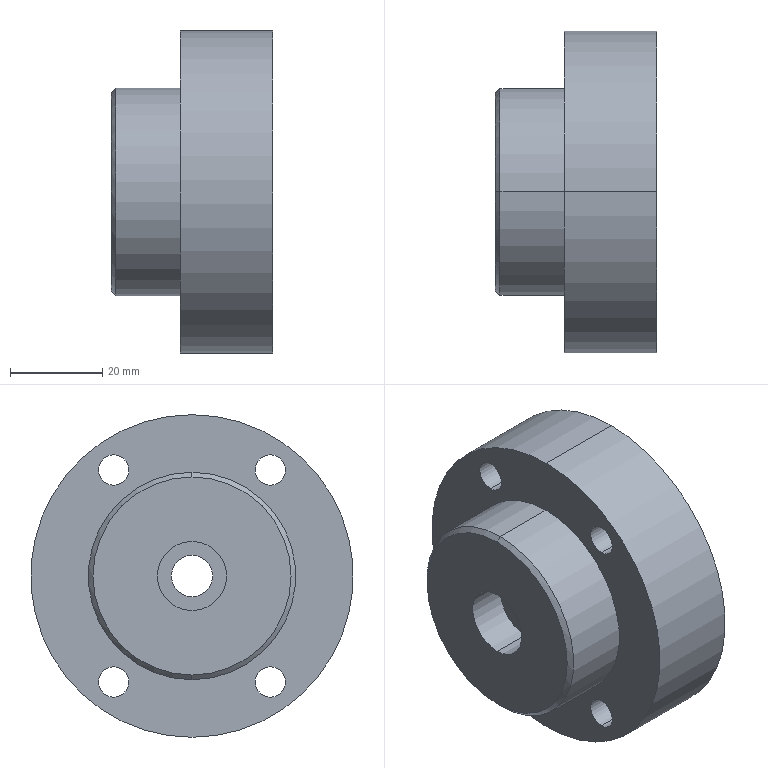Part | SolidWorks | features BaseBody 1 | 1 solid | 39 faces | box 35 x 70 x 70 mm | volume 84677 mm3 | cylinder 26 | plane 9 | cone 4 | commonest cylinder face diameters 6.6 x8 11 x8 9 x2 15 x2 25 x2 45 x2
STEP:
#1=CARTESIAN_POINT('',(8.6,0.,-7.5));
#2=VERTEX_POINT('',#1);
#3=CARTESIAN_POINT('',(8.6,0.,7.5));
#4=VERTEX_POINT('',#3);
#5=CARTESIAN_POINT('',(8.6,0.,0.));
#6=DIRECTION('',(-1.,0.,0.));
#7=DIRECTION('',(0.,0.,1.));
#8=AXIS2_PLACEMENT_3D('',#5,#6,#7);
#9=CIRCLE('',#8,7.5);
#10=EDGE_CURVE('',#2,#4,#9,.T.);
#11=ORIENTED_EDGE('',*,*,#10,.F.);
#12=CARTESIAN_POINT('',(0.,0.,-7.5));
#13=VERTEX_POINT('',#12);
#14=CARTESIAN_POINT('',(0.,0.,-7.5));
#15=DIRECTION('',(-1.,0.,0.));
#16=VECTOR('',#15,1000.);
#17=LINE('',#14,#16);
#18=EDGE_CURVE('',#2,#13,#17,.T.);
#19=ORIENTED_EDGE('',*,*,#18,.T.);
#20=CARTESIAN_POINT('',(0.,0.,7.5));
#21=VERTEX_POINT('',#20);
#22=CARTESIAN_POINT('',(0.,0.,0.));
#23=DIRECTION('',(-1.,0.,0.));
#24=DIRECTION('',(0.,0.,1.));
#25=AXIS2_PLACEMENT_3D('',#22,#23,#24);
#26=CIRCLE('',#25,7.5);
#27=EDGE_CURVE('',#13,#21,#26,.T.);
#28=ORIENTED_EDGE('',*,*,#27,.T.);
#29=CARTESIAN_POINT('',(0.,0.,7.5));
#30=DIRECTION('',(-1.,0.,0.));
#31=VECTOR('',#30,1000.);
#32=LINE('',#29,#31);
#33=EDGE_CURVE('',#4,#21,#32,.T.);
#34=ORIENTED_EDGE('',*,*,#33,.F.);
#35=EDGE_LOOP('',(#11,#19,#28,#34));
#36=FACE_OUTER_BOUND('',#35,.T.);
#37=CARTESIAN_POINT('',(0.,0.,0.));
#38=DIRECTION('',(-1.,0.,0.));
#39=DIRECTION('',(0.,0.,1.));
#40=AXIS2_PLACEMENT_3D('',#37,#38,#39);
#41=CYLINDRICAL_SURFACE('',#40,7.5);
#42=ADVANCED_FACE('',(#36),#41,.F.);
#43=CARTESIAN_POINT('',(15.,0.,-4.5));
#44=VERTEX_POINT('',#43);
#45=CARTESIAN_POINT('',(15.,0.,4.5));
#46=VERTEX_POINT('',#45);
#47=CARTESIAN_POINT('',(15.,0.,0.));
#48=DIRECTION('',(-1.,0.,0.));
#49=DIRECTION('',(0.,0.,1.));
#50=AXIS2_PLACEMENT_3D('',#47,#48,#49);
#51=CIRCLE('',#50,4.5);
#52=EDGE_CURVE('',#44,#46,#51,.T.);
#53=ORIENTED_EDGE('',*,*,#52,.F.);
#54=CARTESIAN_POINT('',(8.6,0.,-4.5));
#55=VERTEX_POINT('',#54);
#56=CARTESIAN_POINT('',(0.,0.,-4.5));
#57=DIRECTION('',(-1.,0.,0.));
#58=VECTOR('',#57,1000.);
#59=LINE('',#56,#58);
#60=EDGE_CURVE('',#44,#55,#59,.T.);
#61=ORIENTED_EDGE('',*,*,#60,.T.);
#62=CARTESIAN_POINT('',(8.6,0.,4.5));
#63=VERTEX_POINT('',#62);
#64=CARTESIAN_POINT('',(8.6,0.,0.));
#65=DIRECTION('',(-1.,0.,0.));
#66=DIRECTION('',(0.,0.,1.));
#67=AXIS2_PLACEMENT_3D('',#64,#65,#66);
#68=CIRCLE('',#67,4.5);
#69=EDGE_CURVE('',#55,#63,#68,.T.);
#70=ORIENTED_EDGE('',*,*,#69,.T.);
#71=CARTESIAN_POINT('',(0.,0.,4.5));
#72=DIRECTION('',(-1.,0.,0.));
#73=VECTOR('',#72,1000.);
#74=LINE('',#71,#73);
#75=EDGE_CURVE('',#46,#63,#74,.T.);
#76=ORIENTED_EDGE('',*,*,#75,.F.);
#77=EDGE_LOOP('',(#53,#61,#70,#76));
#78=FACE_OUTER_BOUND('',#77,.T.);
#79=CARTESIAN_POINT('',(0.,0.,0.));
#80=DIRECTION('',(-1.,0.,0.));
#81=DIRECTION('',(0.,0.,1.));
#82=AXIS2_PLACEMENT_3D('',#79,#80,#81);
#83=CYLINDRICAL_SURFACE('',#82,4.5);
#84=ADVANCED_FACE('',(#78),#83,.F.);
#85=CARTESIAN_POINT('',(0.,0.,21.5));
#86=VERTEX_POINT('',#85);
#87=CARTESIAN_POINT('',(0.,0.,-21.5));
#88=VERTEX_POINT('',#87);
#89=CARTESIAN_POINT('',(0.,0.,0.));
#90=DIRECTION('',(-1.,0.,0.));
#91=DIRECTION('',(0.,0.,-1.));
#92=AXIS2_PLACEMENT_3D('',#89,#90,#91);
#93=CIRCLE('',#92,21.5);
#94=EDGE_CURVE('',#86,#88,#93,.T.);
#95=ORIENTED_EDGE('',*,*,#94,.F.);
#96=CARTESIAN_POINT('',(1.,0.,22.5));
#97=VERTEX_POINT('',#96);
#98=CARTESIAN_POINT('',(1.,0.,22.5));
#99=DIRECTION('',(0.7071,0.,0.7071));
#100=VECTOR('',#99,1000.);
#101=LINE('',#98,#100);
#102=EDGE_CURVE('',#86,#97,#101,.T.);
#103=ORIENTED_EDGE('',*,*,#102,.T.);
#104=CARTESIAN_POINT('',(1.,0.,-22.5));
#105=VERTEX_POINT('',#104);
#106=CARTESIAN_POINT('',(1.,0.,0.));
#107=DIRECTION('',(1.,0.,0.));
#108=DIRECTION('',(0.,0.,-1.));
#109=AXIS2_PLACEMENT_3D('',#106,#107,#108);
#110=CIRCLE('',#109,22.5);
#111=EDGE_CURVE('',#105,#97,#110,.T.);
#112=ORIENTED_EDGE('',*,*,#111,.F.);
#113=CARTESIAN_POINT('',(1.,0.,-22.5));
#114=DIRECTION('',(0.7071,0.,-0.7071));
#115=VECTOR('',#114,1000.);
#116=LINE('',#113,#115);
#117=EDGE_CURVE('',#88,#105,#116,.T.);
#118=ORIENTED_EDGE('',*,*,#117,.F.);
#119=EDGE_LOOP('',(#95,#103,#112,#118));
#120=FACE_OUTER_BOUND('',#119,.T.);
#121=CARTESIAN_POINT('',(1.,0.,0.));
#122=DIRECTION('',(1.,0.,0.));
#123=DIRECTION('',(0.,0.,-1.));
#124=AXIS2_PLACEMENT_3D('',#121,#122,#123);
#125=CONICAL_SURFACE('',#124,22.5,0.7854);
#126=ADVANCED_FACE('',(#120),#125,.T.);
#127=CARTESIAN_POINT('',(34.,0.,12.5));
#128=VERTEX_POINT('',#127);
#129=CARTESIAN_POINT('',(34.,0.,-12.5));
#130=VERTEX_POINT('',#129);
#131=CARTESIAN_POINT('',(34.,0.,0.));
#132=DIRECTION('',(1.,0.,0.));
#133=DIRECTION('',(0.,0.,-1.));
#134=AXIS2_PLACEMENT_3D('',#131,#132,#133);
#135=CIRCLE('',#134,12.5);
#136=EDGE_CURVE('',#128,#130,#135,.T.);
#137=ORIENTED_EDGE('',*,*,#136,.F.);
#138=CARTESIAN_POINT('',(35.,0.,13.5));
#139=VERTEX_POINT('',#138);
#140=CARTESIAN_POINT('',(35.,0.,13.5));
#141=DIRECTION('',(0.7071,0.,0.7071));
#142=VECTOR('',#141,1000.);
#143=LINE('',#140,#142);
#144=EDGE_CURVE('',#128,#139,#143,.T.);
#145=ORIENTED_EDGE('',*,*,#144,.T.);
#146=CARTESIAN_POINT('',(35.,0.,-13.5));
#147=VERTEX_POINT('',#146);
#148=CARTESIAN_POINT('',(35.,0.,0.));
#149=DIRECTION('',(-1.,0.,0.));
#150=DIRECTION('',(0.,0.,-1.));
#151=AXIS2_PLACEMENT_3D('',#148,#149,#150);
#152=CIRCLE('',#151,13.5);
#153=EDGE_CURVE('',#147,#139,#152,.T.);
#154=ORIENTED_EDGE('',*,*,#153,.F.);
#155=CARTESIAN_POINT('',(35.,0.,-13.5));
#156=DIRECTION('',(0.7071,0.,-0.7071));
#157=VECTOR('',#156,1000.);
#158=LINE('',#155,#157);
#159=EDGE_CURVE('',#130,#147,#158,.T.);
#160=ORIENTED_EDGE('',*,*,#159,.F.);
#161=EDGE_LOOP('',(#137,#145,#154,#160));
#162=FACE_OUTER_BOUND('',#161,.T.);
#163=CARTESIAN_POINT('',(35.,0.,0.));
#164=DIRECTION('',(1.,0.,0.));
#165=DIRECTION('',(0.,0.,-1.));
#166=AXIS2_PLACEMENT_3D('',#163,#164,#165);
#167=CONICAL_SURFACE('',#166,13.5,0.7854);
#168=ADVANCED_FACE('',(#162),#167,.F.);
#169=CARTESIAN_POINT('',(28.6,17.,28.5));
#170=VERTEX_POINT('',#169);
#171=CARTESIAN_POINT('',(28.6,17.,17.5));
#172=VERTEX_POINT('',#171);
#173=CARTESIAN_POINT('',(28.6,17.,23.));
#174=DIRECTION('',(1.,0.,0.));
#175=DIRECTION('',(0.,0.,-1.));
#176=AXIS2_PLACEMENT_3D('',#173,#174,#175);
#177=CIRCLE('',#176,5.5);
#178=EDGE_CURVE('',#170,#172,#177,.T.);
#179=ORIENTED_EDGE('',*,*,#178,.F.);
#180=CARTESIAN_POINT('',(35.,17.,28.5));
#181=VERTEX_POINT('',#180);
#182=CARTESIAN_POINT('',(35.,17.,28.5));
#183=DIRECTION('',(1.,0.,0.));
#184=VECTOR('',#183,1000.);
#185=LINE('',#182,#184);
#186=EDGE_CURVE('',#170,#181,#185,.T.);
#187=ORIENTED_EDGE('',*,*,#186,.T.);
#188=CARTESIAN_POINT('',(35.,17.,17.5));
#189=VERTEX_POINT('',#188);
#190=CARTESIAN_POINT('',(35.,17.,23.));
#191=DIRECTION('',(1.,0.,0.));
#192=DIRECTION('',(0.,0.,-1.));
#193=AXIS2_PLACEMENT_3D('',#190,#191,#192);
#194=CIRCLE('',#193,5.5);
#195=EDGE_CURVE('',#181,#189,#194,.T.);
#196=ORIENTED_EDGE('',*,*,#195,.T.);
#197=CARTESIAN_POINT('',(35.,17.,17.5));
#198=DIRECTION('',(1.,0.,0.));
#199=VECTOR('',#198,1000.);
#200=LINE('',#197,#199);
#201=EDGE_CURVE('',#172,#189,#200,.T.);
#202=ORIENTED_EDGE('',*,*,#201,.F.);
#203=EDGE_LOOP('',(#179,#187,#196,#202));
#204=FACE_OUTER_BOUND('',#203,.T.);
#205=CARTESIAN_POINT('',(35.,17.,23.));
#206=DIRECTION('',(1.,0.,0.));
#207=DIRECTION('',(0.,0.,-1.));
#208=AXIS2_PLACEMENT_3D('',#205,#206,#207);
#209=CYLINDRICAL_SURFACE('',#208,5.5);
#210=ADVANCED_FACE('',(#204),#209,.F.);
#211=CARTESIAN_POINT('',(15.,17.,26.3));
#212=VERTEX_POINT('',#211);
#213=CARTESIAN_POINT('',(15.,17.,19.7));
#214=VERTEX_POINT('',#213);
#215=CARTESIAN_POINT('',(15.,17.,23.));
#216=DIRECTION('',(1.,0.,0.));
#217=DIRECTION('',(0.,0.,-1.));
#218=AXIS2_PLACEMENT_3D('',#215,#216,#217);
#219=CIRCLE('',#218,3.3);
#220=EDGE_CURVE('',#212,#214,#219,.T.);
#221=ORIENTED_EDGE('',*,*,#220,.F.);
#222=CARTESIAN_POINT('',(28.6,17.,26.3));
#223=VERTEX_POINT('',#222);
#224=CARTESIAN_POINT('',(35.,17.,26.3));
#225=DIRECTION('',(1.,0.,0.));
#226=VECTOR('',#225,1000.);
#227=LINE('',#224,#226);
#228=EDGE_CURVE('',#212,#223,#227,.T.);
#229=ORIENTED_EDGE('',*,*,#228,.T.);
#230=CARTESIAN_POINT('',(28.6,17.,19.7));
#231=VERTEX_POINT('',#230);
#232=CARTESIAN_POINT('',(28.6,17.,23.));
#233=DIRECTION('',(1.,0.,0.));
#234=DIRECTION('',(0.,0.,-1.));
#235=AXIS2_PLACEMENT_3D('',#232,#233,#234);
#236=CIRCLE('',#235,3.3);
#237=EDGE_CURVE('',#223,#231,#236,.T.);
#238=ORIENTED_EDGE('',*,*,#237,.T.);
#239=CARTESIAN_POINT('',(35.,17.,19.7));
#240=DIRECTION('',(1.,0.,0.));
#241=VECTOR('',#240,1000.);
#242=LINE('',#239,#241);
#243=EDGE_CURVE('',#214,#231,#242,.T.);
#244=ORIENTED_EDGE('',*,*,#243,.F.);
#245=EDGE_LOOP('',(#221,#229,#238,#244));
#246=FACE_OUTER_BOUND('',#245,.T.);
#247=CARTESIAN_POINT('',(35.,17.,23.));
#248=DIRECTION('',(1.,0.,0.));
#249=DIRECTION('',(0.,0.,-1.));
#250=AXIS2_PLACEMENT_3D('',#247,#248,#249);
#251=CYLINDRICAL_SURFACE('',#250,3.3);
#252=ADVANCED_FACE('',(#246),#251,.F.);
#253=CARTESIAN_POINT('',(28.6,17.,-17.5));
#254=VERTEX_POINT('',#253);
#255=CARTESIAN_POINT('',(28.6,17.,-28.5));
#256=VERTEX_POINT('',#255);
#257=CARTESIAN_POINT('',(28.6,17.,-23.));
#258=DIRECTION('',(1.,0.,0.));
#259=DIRECTION('',(0.,0.,-1.));
#260=AXIS2_PLACEMENT_3D('',#257,#258,#259);
#261=CIRCLE('',#260,5.5);
#262=EDGE_CURVE('',#254,#256,#261,.T.);
#263=ORIENTED_EDGE('',*,*,#262,.F.);
#264=CARTESIAN_POINT('',(35.,17.,-17.5));
#265=VERTEX_POINT('',#264);
#266=CARTESIAN_POINT('',(35.,17.,-17.5));
#267=DIRECTION('',(1.,0.,0.));
#268=VECTOR('',#267,1000.);
#269=LINE('',#266,#268);
#270=EDGE_CURVE('',#254,#265,#269,.T.);
#271=ORIENTED_EDGE('',*,*,#270,.T.);
#272=CARTESIAN_POINT('',(35.,17.,-28.5));
#273=VERTEX_POINT('',#272);
#274=CARTESIAN_POINT('',(35.,17.,-23.));
#275=DIRECTION('',(1.,0.,0.));
#276=DIRECTION('',(0.,0.,-1.));
#277=AXIS2_PLACEMENT_3D('',#274,#275,#276);
#278=CIRCLE('',#277,5.5);
#279=EDGE_CURVE('',#265,#273,#278,.T.);
#280=ORIENTED_EDGE('',*,*,#279,.T.);
#281=CARTESIAN_POINT('',(35.,17.,-28.5));
#282=DIRECTION('',(1.,0.,0.));
#283=VECTOR('',#282,1000.);
#284=LINE('',#281,#283);
#285=EDGE_CURVE('',#256,#273,#284,.T.);
#286=ORIENTED_EDGE('',*,*,#285,.F.);
#287=EDGE_LOOP('',(#263,#271,#280,#286));
#288=FACE_OUTER_BOUND('',#287,.T.);
#289=CARTESIAN_POINT('',(35.,17.,-23.));
#290=DIRECTION('',(1.,0.,0.));
#291=DIRECTION('',(0.,0.,-1.));
#292=AXIS2_PLACEMENT_3D('',#289,#290,#291);
#293=CYLINDRICAL_SURFACE('',#292,5.5);
#294=ADVANCED_FACE('',(#288),#293,.F.);
#295=CARTESIAN_POINT('',(15.,17.,-19.7));
#296=VERTEX_POINT('',#295);
#297=CARTESIAN_POINT('',(15.,17.,-26.3));
#298=VERTEX_POINT('',#297);
#299=CARTESIAN_POINT('',(15.,17.,-23.));
#300=DIRECTION('',(1.,0.,0.));
#301=DIRECTION('',(0.,0.,-1.));
#302=AXIS2_PLACEMENT_3D('',#299,#300,#301);
#303=CIRCLE('',#302,3.3);
#304=EDGE_CURVE('',#296,#298,#303,.T.);
#305=ORIENTED_EDGE('',*,*,#304,.F.);
#306=CARTESIAN_POINT('',(28.6,17.,-19.7));
#307=VERTEX_POINT('',#306);
#308=CARTESIAN_POINT('',(35.,17.,-19.7));
#309=DIRECTION('',(1.,0.,0.));
#310=VECTOR('',#309,1000.);
#311=LINE('',#308,#310);
#312=EDGE_CURVE('',#296,#307,#311,.T.);
#313=ORIENTED_EDGE('',*,*,#312,.T.);
#314=CARTESIAN_POINT('',(28.6,17.,-26.3));
#315=VERTEX_POINT('',#314);
#316=CARTESIAN_POINT('',(28.6,17.,-23.));
#317=DIRECTION('',(1.,0.,0.));
#318=DIRECTION('',(0.,0.,-1.));
#319=AXIS2_PLACEMENT_3D('',#316,#317,#318);
#320=CIRCLE('',#319,3.3);
#321=EDGE_CURVE('',#307,#315,#320,.T.);
#322=ORIENTED_EDGE('',*,*,#321,.T.);
#323=CARTESIAN_POINT('',(35.,17.,-26.3));
#324=DIRECTION('',(1.,0.,0.));
#325=VECTOR('',#324,1000.);
#326=LINE('',#323,#325);
#327=EDGE_CURVE('',#298,#315,#326,.T.);
#328=ORIENTED_EDGE('',*,*,#327,.F.);
#329=EDGE_LOOP('',(#305,#313,#322,#328));
#330=FACE_OUTER_BOUND('',#329,.T.);
#331=CARTESIAN_POINT('',(35.,17.,-23.));
#332=DIRECTION('',(1.,0.,0.));
#333=DIRECTION('',(0.,0.,-1.));
#334=AXIS2_PLACEMENT_3D('',#331,#332,#333);
#335=CYLINDRICAL_SURFACE('',#334,3.3);
#336=ADVANCED_FACE('',(#330),#335,.F.);
#337=CARTESIAN_POINT('',(28.6,-17.,-17.5));
#338=VERTEX_POINT('',#337);
#339=CARTESIAN_POINT('',(28.6,-17.,-28.5));
#340=VERTEX_POINT('',#339);
#341=CARTESIAN_POINT('',(28.6,-17.,-23.));
#342=DIRECTION('',(1.,0.,0.));
#343=DIRECTION('',(0.,0.,-1.));
#344=AXIS2_PLACEMENT_3D('',#341,#342,#343);
#345=CIRCLE('',#344,5.5);
#346=EDGE_CURVE('',#338,#340,#345,.T.);
#347=ORIENTED_EDGE('',*,*,#346,.F.);
#348=CARTESIAN_POINT('',(35.,-17.,-17.5));
#349=VERTEX_POINT('',#348);
#350=CARTESIAN_POINT('',(35.,-17.,-17.5));
#351=DIRECTION('',(1.,0.,0.));
#352=VECTOR('',#351,1000.);
#353=LINE('',#350,#352);
#354=EDGE_CURVE('',#338,#349,#353,.T.);
#355=ORIENTED_EDGE('',*,*,#354,.T.);
#356=CARTESIAN_POINT('',(35.,-17.,-28.5));
#357=VERTEX_POINT('',#356);
#358=CARTESIAN_POINT('',(35.,-17.,-23.));
#359=DIRECTION('',(1.,0.,0.));
#360=DIRECTION('',(0.,0.,-1.));
#361=AXIS2_PLACEMENT_3D('',#358,#359,#360);
#362=CIRCLE('',#361,5.5);
#363=EDGE_CURVE('',#349,#357,#362,.T.);
#364=ORIENTED_EDGE('',*,*,#363,.T.);
#365=CARTESIAN_POINT('',(35.,-17.,-28.5));
#366=DIRECTION('',(1.,0.,0.));
#367=VECTOR('',#366,1000.);
#368=LINE('',#365,#367);
#369=EDGE_CURVE('',#340,#357,#368,.T.);
#370=ORIENTED_EDGE('',*,*,#369,.F.);
#371=EDGE_LOOP('',(#347,#355,#364,#370));
#372=FACE_OUTER_BOUND('',#371,.T.);
#373=CARTESIAN_POINT('',(35.,-17.,-23.));
#374=DIRECTION('',(1.,0.,0.));
#375=DIRECTION('',(0.,0.,-1.));
#376=AXIS2_PLACEMENT_3D('',#373,#374,#375);
#377=CYLINDRICAL_SURFACE('',#376,5.5);
#378=ADVANCED_FACE('',(#372),#377,.F.);
#379=CARTESIAN_POINT('',(15.,-17.,-19.7));
#380=VERTEX_POINT('',#379);
#381=CARTESIAN_POINT('',(15.,-17.,-26.3));
#382=VERTEX_POINT('',#381);
#383=CARTESIAN_POINT('',(15.,-17.,-23.));
#384=DIRECTION('',(1.,0.,0.));
#385=DIRECTION('',(0.,0.,-1.));
#386=AXIS2_PLACEMENT_3D('',#383,#384,#385);
#387=CIRCLE('',#386,3.3);
#388=EDGE_CURVE('',#380,#382,#387,.T.);
#389=ORIENTED_EDGE('',*,*,#388,.F.);
#390=CARTESIAN_POINT('',(28.6,-17.,-19.7));
#391=VERTEX_POINT('',#390);
#392=CARTESIAN_POINT('',(35.,-17.,-19.7));
#393=DIRECTION('',(1.,0.,0.));
#394=VECTOR('',#393,1000.);
#395=LINE('',#392,#394);
#396=EDGE_CURVE('',#380,#391,#395,.T.);
#397=ORIENTED_EDGE('',*,*,#396,.T.);
#398=CARTESIAN_POINT('',(28.6,-17.,-26.3));
#399=VERTEX_POINT('',#398);
#400=CARTESIAN_POINT('',(28.6,-17.,-23.));
#401=DIRECTION('',(1.,0.,0.));
#402=DIRECTION('',(0.,0.,-1.));
#403=AXIS2_PLACEMENT_3D('',#400,#401,#402);
#404=CIRCLE('',#403,3.3);
#405=EDGE_CURVE('',#391,#399,#404,.T.);
#406=ORIENTED_EDGE('',*,*,#405,.T.);
#407=CARTESIAN_POINT('',(35.,-17.,-26.3));
#408=DIRECTION('',(1.,0.,0.));
#409=VECTOR('',#408,1000.);
#410=LINE('',#407,#409);
#411=EDGE_CURVE('',#382,#399,#410,.T.);
#412=ORIENTED_EDGE('',*,*,#411,.F.);
#413=EDGE_LOOP('',(#389,#397,#406,#412));
#414=FACE_OUTER_BOUND('',#413,.T.);
#415=CARTESIAN_POINT('',(35.,-17.,-23.));
#416=DIRECTION('',(1.,0.,0.));
#417=DIRECTION('',(0.,0.,-1.));
#418=AXIS2_PLACEMENT_3D('',#415,#416,#417);
#419=CYLINDRICAL_SURFACE('',#418,3.3);
#420=ADVANCED_FACE('',(#414),#419,.F.);
#421=CARTESIAN_POINT('',(28.6,-17.,28.5));
#422=VERTEX_POINT('',#421);
#423=CARTESIAN_POINT('',(28.6,-17.,17.5));
#424=VERTEX_POINT('',#423);
#425=CARTESIAN_POINT('',(28.6,-17.,23.));
#426=DIRECTION('',(1.,0.,0.));
#427=DIRECTION('',(0.,0.,-1.));
#428=AXIS2_PLACEMENT_3D('',#425,#426,#427);
#429=CIRCLE('',#428,5.5);
#430=EDGE_CURVE('',#422,#424,#429,.T.);
#431=ORIENTED_EDGE('',*,*,#430,.F.);
#432=CARTESIAN_POINT('',(35.,-17.,28.5));
#433=VERTEX_POINT('',#432);
#434=CARTESIAN_POINT('',(35.,-17.,28.5));
#435=DIRECTION('',(1.,0.,0.));
#436=VECTOR('',#435,1000.);
#437=LINE('',#434,#436);
#438=EDGE_CURVE('',#422,#433,#437,.T.);
#439=ORIENTED_EDGE('',*,*,#438,.T.);
#440=CARTESIAN_POINT('',(35.,-17.,17.5));
#441=VERTEX_POINT('',#440);
#442=CARTESIAN_POINT('',(35.,-17.,23.));
#443=DIRECTION('',(1.,0.,0.));
#444=DIRECTION('',(0.,0.,-1.));
#445=AXIS2_PLACEMENT_3D('',#442,#443,#444);
#446=CIRCLE('',#445,5.5);
#447=EDGE_CURVE('',#433,#441,#446,.T.);
#448=ORIENTED_EDGE('',*,*,#447,.T.);
#449=CARTESIAN_POINT('',(35.,-17.,17.5));
#450=DIRECTION('',(1.,0.,0.));
#451=VECTOR('',#450,1000.);
#452=LINE('',#449,#451);
#453=EDGE_CURVE('',#424,#441,#452,.T.);
#454=ORIENTED_EDGE('',*,*,#453,.F.);
#455=EDGE_LOOP('',(#431,#439,#448,#454));
#456=FACE_OUTER_BOUND('',#455,.T.);
#457=CARTESIAN_POINT('',(35.,-17.,23.));
#458=DIRECTION('',(1.,0.,0.));
#459=DIRECTION('',(0.,0.,-1.));
#460=AXIS2_PLACEMENT_3D('',#457,#458,#459);
#461=CYLINDRICAL_SURFACE('',#460,5.5);
#462=ADVANCED_FACE('',(#456),#461,.F.);
#463=CARTESIAN_POINT('',(15.,-17.,26.3));
#464=VERTEX_POINT('',#463);
#465=CARTESIAN_POINT('',(15.,-17.,19.7));
#466=VERTEX_POINT('',#465);
#467=CARTESIAN_POINT('',(15.,-17.,23.));
#468=DIRECTION('',(1.,0.,0.));
#469=DIRECTION('',(0.,0.,-1.));
#470=AXIS2_PLACEMENT_3D('',#467,#468,#469);
#471=CIRCLE('',#470,3.3);
#472=EDGE_CURVE('',#464,#466,#471,.T.);
#473=ORIENTED_EDGE('',*,*,#472,.F.);
#474=CARTESIAN_POINT('',(28.6,-17.,26.3));
#475=VERTEX_POINT('',#474);
#476=CARTESIAN_POINT('',(35.,-17.,26.3));
#477=DIRECTION('',(1.,0.,0.));
#478=VECTOR('',#477,1000.);
#479=LINE('',#476,#478);
#480=EDGE_CURVE('',#464,#475,#479,.T.);
#481=ORIENTED_EDGE('',*,*,#480,.T.);
#482=CARTESIAN_POINT('',(28.6,-17.,19.7));
#483=VERTEX_POINT('',#482);
#484=CARTESIAN_POINT('',(28.6,-17.,23.));
#485=DIRECTION('',(1.,0.,0.));
#486=DIRECTION('',(0.,0.,-1.));
#487=AXIS2_PLACEMENT_3D('',#484,#485,#486);
#488=CIRCLE('',#487,3.3);
#489=EDGE_CURVE('',#475,#483,#488,.T.);
#490=ORIENTED_EDGE('',*,*,#489,.T.);
#491=CARTESIAN_POINT('',(35.,-17.,19.7));
#492=DIRECTION('',(1.,0.,0.));
#493=VECTOR('',#492,1000.);
#494=LINE('',#491,#493);
#495=EDGE_CURVE('',#466,#483,#494,.T.);
#496=ORIENTED_EDGE('',*,*,#495,.F.);
#497=EDGE_LOOP('',(#473,#481,#490,#496));
#498=FACE_OUTER_BOUND('',#497,.T.);
#499=CARTESIAN_POINT('',(35.,-17.,23.));
#500=DIRECTION('',(1.,0.,0.));
#501=DIRECTION('',(0.,0.,-1.));
#502=AXIS2_PLACEMENT_3D('',#499,#500,#501);
#503=CYLINDRICAL_SURFACE('',#502,3.3);
#504=ADVANCED_FACE('',(#498),#503,.F.);
#505=CARTESIAN_POINT('',(15.,0.,-12.5));
#506=VERTEX_POINT('',#505);
#507=CARTESIAN_POINT('',(15.,0.,12.5));
#508=VERTEX_POINT('',#507);
#509=CARTESIAN_POINT('',(15.,0.,0.));
#510=DIRECTION('',(-1.,0.,0.));
#511=DIRECTION('',(0.,0.,1.));
#512=AXIS2_PLACEMENT_3D('',#509,#510,#511);
#513=CIRCLE('',#512,12.5);
#514=EDGE_CURVE('',#506,#508,#513,.T.);
#515=ORIENTED_EDGE('',*,*,#514,.T.);
#516=CARTESIAN_POINT('',(15.,0.,12.5));
#517=DIRECTION('',(1.,0.,0.));
#518=VECTOR('',#517,1000.);
#519=LINE('',#516,#518);
#520=EDGE_CURVE('',#508,#128,#519,.T.);
#521=ORIENTED_EDGE('',*,*,#520,.T.);
#522=ORIENTED_EDGE('',*,*,#136,.T.);
#523=CARTESIAN_POINT('',(15.,0.,-12.5));
#524=DIRECTION('',(1.,0.,0.));
#525=VECTOR('',#524,1000.);
#526=LINE('',#523,#525);
#527=EDGE_CURVE('',#506,#130,#526,.T.);
#528=ORIENTED_EDGE('',*,*,#527,.F.);
#529=EDGE_LOOP('',(#515,#521,#522,#528));
#530=FACE_OUTER_BOUND('',#529,.T.);
#531=CARTESIAN_POINT('',(15.,0.,0.));
#532=DIRECTION('',(1.,0.,0.));
#533=DIRECTION('',(0.,0.,-1.));
#534=AXIS2_PLACEMENT_3D('',#531,#532,#533);
#535=CYLINDRICAL_SURFACE('',#534,12.5);
#536=ADVANCED_FACE('',(#530),#535,.F.);
#537=CARTESIAN_POINT('',(35.,0.,-35.));
#538=VERTEX_POINT('',#537);
#539=CARTESIAN_POINT('',(35.,0.,35.));
#540=VERTEX_POINT('',#539);
#541=CARTESIAN_POINT('',(35.,0.,0.));
#542=DIRECTION('',(1.,0.,0.));
#543=DIRECTION('',(0.,0.,-1.));
#544=AXIS2_PLACEMENT_3D('',#541,#542,#543);
#545=CIRCLE('',#544,35.);
#546=EDGE_CURVE('',#538,#540,#545,.T.);
#547=ORIENTED_EDGE('',*,*,#546,.F.);
#548=CARTESIAN_POINT('',(15.,0.,-35.));
#549=VERTEX_POINT('',#548);
#550=CARTESIAN_POINT('',(35.,0.,-35.));
#551=DIRECTION('',(-1.,0.,0.));
#552=VECTOR('',#551,1000.);
#553=LINE('',#550,#552);
#554=EDGE_CURVE('',#538,#549,#553,.T.);
#555=ORIENTED_EDGE('',*,*,#554,.T.);
#556=CARTESIAN_POINT('',(15.,0.,35.));
#557=VERTEX_POINT('',#556);
#558=CARTESIAN_POINT('',(15.,0.,0.));
#559=DIRECTION('',(1.,0.,0.));
#560=DIRECTION('',(0.,0.,-1.));
#561=AXIS2_PLACEMENT_3D('',#558,#559,#560);
#562=CIRCLE('',#561,35.);
#563=EDGE_CURVE('',#549,#557,#562,.T.);
#564=ORIENTED_EDGE('',*,*,#563,.T.);
#565=CARTESIAN_POINT('',(35.,0.,35.));
#566=DIRECTION('',(-1.,0.,0.));
#567=VECTOR('',#566,1000.);
#568=LINE('',#565,#567);
#569=EDGE_CURVE('',#540,#557,#568,.T.);
#570=ORIENTED_EDGE('',*,*,#569,.F.);
#571=EDGE_LOOP('',(#547,#555,#564,#570));
#572=FACE_OUTER_BOUND('',#571,.T.);
#573=CARTESIAN_POINT('',(35.,0.,0.));
#574=DIRECTION('',(-1.,0.,0.));
#575=DIRECTION('',(0.,0.,1.));
#576=AXIS2_PLACEMENT_3D('',#573,#574,#575);
#577=CYLINDRICAL_SURFACE('',#576,35.);
#578=ADVANCED_FACE('',(#572),#577,.T.);
#579=CARTESIAN_POINT('',(15.,0.,-22.5));
#580=VERTEX_POINT('',#579);
#581=CARTESIAN_POINT('',(15.,0.,22.5));
#582=VERTEX_POINT('',#581);
#583=CARTESIAN_POINT('',(15.,0.,0.));
#584=DIRECTION('',(1.,0.,0.));
#585=DIRECTION('',(0.,0.,-1.));
#586=AXIS2_PLACEMENT_3D('',#583,#584,#585);
#587=CIRCLE('',#586,22.5);
#588=EDGE_CURVE('',#580,#582,#587,.T.);
#589=ORIENTED_EDGE('',*,*,#588,.F.);
#590=CARTESIAN_POINT('',(15.,0.,-22.5));
#591=DIRECTION('',(-1.,0.,0.));
#592=VECTOR('',#591,1000.);
#593=LINE('',#590,#592);
#594=EDGE_CURVE('',#580,#105,#593,.T.);
#595=ORIENTED_EDGE('',*,*,#594,.T.);
#596=ORIENTED_EDGE('',*,*,#111,.T.);
#597=CARTESIAN_POINT('',(15.,0.,22.5));
#598=DIRECTION('',(-1.,0.,0.));
#599=VECTOR('',#598,1000.);
#600=LINE('',#597,#599);
#601=EDGE_CURVE('',#582,#97,#600,.T.);
#602=ORIENTED_EDGE('',*,*,#601,.F.);
#603=EDGE_LOOP('',(#589,#595,#596,#602));
#604=FACE_OUTER_BOUND('',#603,.T.);
#605=CARTESIAN_POINT('',(15.,0.,0.));
#606=DIRECTION('',(-1.,0.,0.));
#607=DIRECTION('',(0.,0.,1.));
#608=AXIS2_PLACEMENT_3D('',#605,#606,#607);
#609=CYLINDRICAL_SURFACE('',#608,22.5);
#610=ADVANCED_FACE('',(#604),#609,.T.);
#611=ORIENTED_EDGE('',*,*,#153,.T.);
#612=CARTESIAN_POINT('',(35.,0.,0.));
#613=DIRECTION('',(-1.,0.,0.));
#614=DIRECTION('',(0.,0.,-1.));
#615=AXIS2_PLACEMENT_3D('',#612,#613,#614);
#616=CIRCLE('',#615,13.5);
#617=EDGE_CURVE('',#139,#147,#616,.T.);
#618=ORIENTED_EDGE('',*,*,#617,.T.);
#619=EDGE_LOOP('',(#611,#618));
#620=FACE_BOUND('',#619,.T.);
#621=CARTESIAN_POINT('',(35.,17.,23.));
#622=DIRECTION('',(1.,0.,0.));
#623=DIRECTION('',(0.,0.,-1.));
#624=AXIS2_PLACEMENT_3D('',#621,#622,#623);
#625=CIRCLE('',#624,5.5);
#626=EDGE_CURVE('',#189,#181,#625,.T.);
#627=ORIENTED_EDGE('',*,*,#626,.F.);
#628=ORIENTED_EDGE('',*,*,#195,.F.);
#629=EDGE_LOOP('',(#627,#628));
#630=FACE_BOUND('',#629,.T.);
#631=CARTESIAN_POINT('',(35.,17.,-23.));
#632=DIRECTION('',(1.,0.,0.));
#633=DIRECTION('',(0.,0.,-1.));
#634=AXIS2_PLACEMENT_3D('',#631,#632,#633);
#635=CIRCLE('',#634,5.5);
#636=EDGE_CURVE('',#273,#265,#635,.T.);
#637=ORIENTED_EDGE('',*,*,#636,.F.);
#638=ORIENTED_EDGE('',*,*,#279,.F.);
#639=EDGE_LOOP('',(#637,#638));
#640=FACE_BOUND('',#639,.T.);
#641=CARTESIAN_POINT('',(35.,-17.,-23.));
#642=DIRECTION('',(1.,0.,0.));
#643=DIRECTION('',(0.,0.,-1.));
#644=AXIS2_PLACEMENT_3D('',#641,#642,#643);
#645=CIRCLE('',#644,5.5);
#646=EDGE_CURVE('',#357,#349,#645,.T.);
#647=ORIENTED_EDGE('',*,*,#646,.F.);
#648=ORIENTED_EDGE('',*,*,#363,.F.);
#649=EDGE_LOOP('',(#647,#648));
#650=FACE_BOUND('',#649,.T.);
#651=CARTESIAN_POINT('',(35.,-17.,23.));
#652=DIRECTION('',(1.,0.,0.));
#653=DIRECTION('',(0.,0.,-1.));
#654=AXIS2_PLACEMENT_3D('',#651,#652,#653);
#655=CIRCLE('',#654,5.5);
#656=EDGE_CURVE('',#441,#433,#655,.T.);
#657=ORIENTED_EDGE('',*,*,#656,.F.);
#658=ORIENTED_EDGE('',*,*,#447,.F.);
#659=EDGE_LOOP('',(#657,#658));
#660=FACE_BOUND('',#659,.T.);
#661=CARTESIAN_POINT('',(35.,0.,0.));
#662=DIRECTION('',(1.,0.,0.));
#663=DIRECTION('',(0.,0.,-1.));
#664=AXIS2_PLACEMENT_3D('',#661,#662,#663);
#665=CIRCLE('',#664,35.);
#666=EDGE_CURVE('',#540,#538,#665,.T.);
#667=ORIENTED_EDGE('',*,*,#666,.T.);
#668=ORIENTED_EDGE('',*,*,#546,.T.);
#669=EDGE_LOOP('',(#667,#668));
#670=FACE_OUTER_BOUND('',#669,.T.);
#671=CARTESIAN_POINT('',(35.,0.,0.));
#672=DIRECTION('',(1.,0.,0.));
#673=DIRECTION('',(0.,0.,-1.));
#674=AXIS2_PLACEMENT_3D('',#671,#672,#673);
#675=PLANE('',#674);
#676=ADVANCED_FACE('',(#620,#630,#640,#650,#660,#670),#675,.T.);
#677=ORIENTED_EDGE('',*,*,#594,.F.);
#678=CARTESIAN_POINT('',(15.,0.,0.));
#679=DIRECTION('',(1.,0.,0.));
#680=DIRECTION('',(0.,0.,-1.));
#681=AXIS2_PLACEMENT_3D('',#678,#679,#680);
#682=CIRCLE('',#681,22.5);
#683=EDGE_CURVE('',#582,#580,#682,.T.);
#684=ORIENTED_EDGE('',*,*,#683,.F.);
#685=ORIENTED_EDGE('',*,*,#601,.T.);
#686=CARTESIAN_POINT('',(1.,0.,0.));
#687=DIRECTION('',(1.,0.,0.));
#688=DIRECTION('',(0.,0.,-1.));
#689=AXIS2_PLACEMENT_3D('',#686,#687,#688);
#690=CIRCLE('',#689,22.5);
#691=EDGE_CURVE('',#97,#105,#690,.T.);
#692=ORIENTED_EDGE('',*,*,#691,.T.);
#693=EDGE_LOOP('',(#677,#684,#685,#692));
#694=FACE_OUTER_BOUND('',#693,.T.);
#695=CARTESIAN_POINT('',(15.,0.,0.));
#696=DIRECTION('',(-1.,0.,0.));
#697=DIRECTION('',(0.,0.,1.));
#698=AXIS2_PLACEMENT_3D('',#695,#696,#697);
#699=CYLINDRICAL_SURFACE('',#698,22.5);
#700=ADVANCED_FACE('',(#694),#699,.T.);
#701=CARTESIAN_POINT('',(0.,0.,0.));
#702=DIRECTION('',(-1.,0.,0.));
#703=DIRECTION('',(0.,0.,1.));
#704=AXIS2_PLACEMENT_3D('',#701,#702,#703);
#705=CIRCLE('',#704,7.5);
#706=EDGE_CURVE('',#21,#13,#705,.T.);
#707=ORIENTED_EDGE('',*,*,#706,.F.);
#708=ORIENTED_EDGE('',*,*,#27,.F.);
#709=EDGE_LOOP('',(#707,#708));
#710=FACE_BOUND('',#709,.T.);
#711=CARTESIAN_POINT('',(0.,0.,0.));
#712=DIRECTION('',(-1.,0.,0.));
#713=DIRECTION('',(0.,0.,-1.));
#714=AXIS2_PLACEMENT_3D('',#711,#712,#713);
#715=CIRCLE('',#714,21.5);
#716=EDGE_CURVE('',#88,#86,#715,.T.);
#717=ORIENTED_EDGE('',*,*,#716,.T.);
#718=ORIENTED_EDGE('',*,*,#94,.T.);
#719=EDGE_LOOP('',(#717,#718));
#720=FACE_OUTER_BOUND('',#719,.T.);
#721=CARTESIAN_POINT('',(0.,0.,0.));
#722=DIRECTION('',(1.,0.,0.));
#723=DIRECTION('',(0.,0.,-1.));
#724=AXIS2_PLACEMENT_3D('',#721,#722,#723);
#725=PLANE('',#724);
#726=ADVANCED_FACE('',(#710,#720),#725,.F.);
#727=CARTESIAN_POINT('',(15.,17.,23.));
#728=DIRECTION('',(1.,0.,0.));
#729=DIRECTION('',(0.,0.,-1.));
#730=AXIS2_PLACEMENT_3D('',#727,#728,#729);
#731=CIRCLE('',#730,3.3);
#732=EDGE_CURVE('',#214,#212,#731,.T.);
#733=ORIENTED_EDGE('',*,*,#732,.T.);
#734=ORIENTED_EDGE('',*,*,#220,.T.);
#735=EDGE_LOOP('',(#733,#734));
#736=FACE_BOUND('',#735,.T.);
#737=CARTESIAN_POINT('',(15.,17.,-23.));
#738=DIRECTION('',(1.,0.,0.));
#739=DIRECTION('',(0.,0.,-1.));
#740=AXIS2_PLACEMENT_3D('',#737,#738,#739);
#741=CIRCLE('',#740,3.3);
#742=EDGE_CURVE('',#298,#296,#741,.T.);
#743=ORIENTED_EDGE('',*,*,#742,.T.);
#744=ORIENTED_EDGE('',*,*,#304,.T.);
#745=EDGE_LOOP('',(#743,#744));
#746=FACE_BOUND('',#745,.T.);
#747=CARTESIAN_POINT('',(15.,-17.,-23.));
#748=DIRECTION('',(1.,0.,0.));
#749=DIRECTION('',(0.,0.,-1.));
#750=AXIS2_PLACEMENT_3D('',#747,#748,#749);
#751=CIRCLE('',#750,3.3);
#752=EDGE_CURVE('',#382,#380,#751,.T.);
#753=ORIENTED_EDGE('',*,*,#752,.T.);
#754=ORIENTED_EDGE('',*,*,#388,.T.);
#755=EDGE_LOOP('',(#753,#754));
#756=FACE_BOUND('',#755,.T.);
#757=CARTESIAN_POINT('',(15.,-17.,23.));
#758=DIRECTION('',(1.,0.,0.));
#759=DIRECTION('',(0.,0.,-1.));
#760=AXIS2_PLACEMENT_3D('',#757,#758,#759);
#761=CIRCLE('',#760,3.3);
#762=EDGE_CURVE('',#466,#464,#761,.T.);
#763=ORIENTED_EDGE('',*,*,#762,.T.);
#764=ORIENTED_EDGE('',*,*,#472,.T.);
#765=EDGE_LOOP('',(#763,#764));
#766=FACE_BOUND('',#765,.T.);
#767=CARTESIAN_POINT('',(15.,0.,0.));
#768=DIRECTION('',(1.,0.,0.));
#769=DIRECTION('',(0.,0.,-1.));
#770=AXIS2_PLACEMENT_3D('',#767,#768,#769);
#771=CIRCLE('',#770,35.);
#772=EDGE_CURVE('',#557,#549,#771,.T.);
#773=ORIENTED_EDGE('',*,*,#772,.F.);
#774=ORIENTED_EDGE('',*,*,#563,.F.);
#775=EDGE_LOOP('',(#773,#774));
#776=FACE_OUTER_BOUND('',#775,.T.);
#777=ORIENTED_EDGE('',*,*,#683,.T.);
#778=ORIENTED_EDGE('',*,*,#588,.T.);
#779=EDGE_LOOP('',(#777,#778));
#780=FACE_BOUND('',#779,.T.);
#781=CARTESIAN_POINT('',(15.,0.,0.));
#782=DIRECTION('',(1.,0.,0.));
#783=DIRECTION('',(0.,0.,-1.));
#784=AXIS2_PLACEMENT_3D('',#781,#782,#783);
#785=PLANE('',#784);
#786=ADVANCED_FACE('',(#736,#746,#756,#766,#776,#780),#785,.F.);
#787=ORIENTED_EDGE('',*,*,#554,.F.);
#788=ORIENTED_EDGE('',*,*,#666,.F.);
#789=ORIENTED_EDGE('',*,*,#569,.T.);
#790=ORIENTED_EDGE('',*,*,#772,.T.);
#791=EDGE_LOOP('',(#787,#788,#789,#790));
#792=FACE_OUTER_BOUND('',#791,.T.);
#793=CARTESIAN_POINT('',(35.,0.,0.));
#794=DIRECTION('',(-1.,0.,0.));
#795=DIRECTION('',(0.,0.,1.));
#796=AXIS2_PLACEMENT_3D('',#793,#794,#795);
#797=CYLINDRICAL_SURFACE('',#796,35.);
#798=ADVANCED_FACE('',(#792),#797,.T.);
#799=ORIENTED_EDGE('',*,*,#520,.F.);
#800=CARTESIAN_POINT('',(15.,0.,0.));
#801=DIRECTION('',(-1.,0.,0.));
#802=DIRECTION('',(0.,0.,1.));
#803=AXIS2_PLACEMENT_3D('',#800,#801,#802);
#804=CIRCLE('',#803,12.5);
#805=EDGE_CURVE('',#508,#506,#804,.T.);
#806=ORIENTED_EDGE('',*,*,#805,.T.);
#807=ORIENTED_EDGE('',*,*,#527,.T.);
#808=CARTESIAN_POINT('',(34.,0.,0.));
#809=DIRECTION('',(1.,0.,0.));
#810=DIRECTION('',(0.,0.,-1.));
#811=AXIS2_PLACEMENT_3D('',#808,#809,#810);
#812=CIRCLE('',#811,12.5);
#813=EDGE_CURVE('',#130,#128,#812,.T.);
#814=ORIENTED_EDGE('',*,*,#813,.T.);
#815=EDGE_LOOP('',(#799,#806,#807,#814));
#816=FACE_OUTER_BOUND('',#815,.T.);
#817=CARTESIAN_POINT('',(15.,0.,0.));
#818=DIRECTION('',(1.,0.,0.));
#819=DIRECTION('',(0.,0.,-1.));
#820=AXIS2_PLACEMENT_3D('',#817,#818,#819);
#821=CYLINDRICAL_SURFACE('',#820,12.5);
#822=ADVANCED_FACE('',(#816),#821,.F.);
#823=CARTESIAN_POINT('',(15.,0.,0.));
#824=DIRECTION('',(-1.,0.,0.));
#825=DIRECTION('',(0.,0.,1.));
#826=AXIS2_PLACEMENT_3D('',#823,#824,#825);
#827=CIRCLE('',#826,4.5);
#828=EDGE_CURVE('',#46,#44,#827,.T.);
#829=ORIENTED_EDGE('',*,*,#828,.T.);
#830=ORIENTED_EDGE('',*,*,#52,.T.);
#831=EDGE_LOOP('',(#829,#830));
#832=FACE_BOUND('',#831,.T.);
#833=ORIENTED_EDGE('',*,*,#514,.F.);
#834=ORIENTED_EDGE('',*,*,#805,.F.);
#835=EDGE_LOOP('',(#833,#834));
#836=FACE_OUTER_BOUND('',#835,.T.);
#837=CARTESIAN_POINT('',(15.,0.,0.));
#838=DIRECTION('',(-1.,0.,0.));
#839=DIRECTION('',(0.,0.,1.));
#840=AXIS2_PLACEMENT_3D('',#837,#838,#839);
#841=PLANE('',#840);
#842=ADVANCED_FACE('',(#832,#836),#841,.F.);
#843=ORIENTED_EDGE('',*,*,#480,.F.);
#844=ORIENTED_EDGE('',*,*,#762,.F.);
#845=ORIENTED_EDGE('',*,*,#495,.T.);
#846=CARTESIAN_POINT('',(28.6,-17.,23.));
#847=DIRECTION('',(1.,0.,0.));
#848=DIRECTION('',(0.,0.,-1.));
#849=AXIS2_PLACEMENT_3D('',#846,#847,#848);
#850=CIRCLE('',#849,3.3);
#851=EDGE_CURVE('',#483,#475,#850,.T.);
#852=ORIENTED_EDGE('',*,*,#851,.T.);
#853=EDGE_LOOP('',(#843,#844,#845,#852));
#854=FACE_OUTER_BOUND('',#853,.T.);
#855=CARTESIAN_POINT('',(35.,-17.,23.));
#856=DIRECTION('',(1.,0.,0.));
#857=DIRECTION('',(0.,0.,-1.));
#858=AXIS2_PLACEMENT_3D('',#855,#856,#857);
#859=CYLINDRICAL_SURFACE('',#858,3.3);
#860=ADVANCED_FACE('',(#854),#859,.F.);
#861=ORIENTED_EDGE('',*,*,#851,.F.);
#862=ORIENTED_EDGE('',*,*,#489,.F.);
#863=EDGE_LOOP('',(#861,#862));
#864=FACE_BOUND('',#863,.T.);
#865=CARTESIAN_POINT('',(28.6,-17.,23.));
#866=DIRECTION('',(1.,0.,0.));
#867=DIRECTION('',(0.,0.,-1.));
#868=AXIS2_PLACEMENT_3D('',#865,#866,#867);
#869=CIRCLE('',#868,5.5);
#870=EDGE_CURVE('',#424,#422,#869,.T.);
#871=ORIENTED_EDGE('',*,*,#870,.T.);
#872=ORIENTED_EDGE('',*,*,#430,.T.);
#873=EDGE_LOOP('',(#871,#872));
#874=FACE_OUTER_BOUND('',#873,.T.);
#875=CARTESIAN_POINT('',(28.6,-13.7,23.));
#876=DIRECTION('',(-1.,0.,0.));
#877=DIRECTION('',(0.,0.,1.));
#878=AXIS2_PLACEMENT_3D('',#875,#876,#877);
#879=PLANE('',#878);
#880=ADVANCED_FACE('',(#864,#874),#879,.F.);
#881=ORIENTED_EDGE('',*,*,#438,.F.);
#882=ORIENTED_EDGE('',*,*,#870,.F.);
#883=ORIENTED_EDGE('',*,*,#453,.T.);
#884=ORIENTED_EDGE('',*,*,#656,.T.);
#885=EDGE_LOOP('',(#881,#882,#883,#884));
#886=FACE_OUTER_BOUND('',#885,.T.);
#887=CARTESIAN_POINT('',(35.,-17.,23.));
#888=DIRECTION('',(1.,0.,0.));
#889=DIRECTION('',(0.,0.,-1.));
#890=AXIS2_PLACEMENT_3D('',#887,#888,#889);
#891=CYLINDRICAL_SURFACE('',#890,5.5);
#892=ADVANCED_FACE('',(#886),#891,.F.);
#893=ORIENTED_EDGE('',*,*,#396,.F.);
#894=ORIENTED_EDGE('',*,*,#752,.F.);
#895=ORIENTED_EDGE('',*,*,#411,.T.);
#896=CARTESIAN_POINT('',(28.6,-17.,-23.));
#897=DIRECTION('',(1.,0.,0.));
#898=DIRECTION('',(0.,0.,-1.));
#899=AXIS2_PLACEMENT_3D('',#896,#897,#898);
#900=CIRCLE('',#899,3.3);
#901=EDGE_CURVE('',#399,#391,#900,.T.);
#902=ORIENTED_EDGE('',*,*,#901,.T.);
#903=EDGE_LOOP('',(#893,#894,#895,#902));
#904=FACE_OUTER_BOUND('',#903,.T.);
#905=CARTESIAN_POINT('',(35.,-17.,-23.));
#906=DIRECTION('',(1.,0.,0.));
#907=DIRECTION('',(0.,0.,-1.));
#908=AXIS2_PLACEMENT_3D('',#905,#906,#907);
#909=CYLINDRICAL_SURFACE('',#908,3.3);
#910=ADVANCED_FACE('',(#904),#909,.F.);
#911=ORIENTED_EDGE('',*,*,#901,.F.);
#912=ORIENTED_EDGE('',*,*,#405,.F.);
#913=EDGE_LOOP('',(#911,#912));
#914=FACE_BOUND('',#913,.T.);
#915=CARTESIAN_POINT('',(28.6,-17.,-23.));
#916=DIRECTION('',(1.,0.,0.));
#917=DIRECTION('',(0.,0.,-1.));
#918=AXIS2_PLACEMENT_3D('',#915,#916,#917);
#919=CIRCLE('',#918,5.5);
#920=EDGE_CURVE('',#340,#338,#919,.T.);
#921=ORIENTED_EDGE('',*,*,#920,.T.);
#922=ORIENTED_EDGE('',*,*,#346,.T.);
#923=EDGE_LOOP('',(#921,#922));
#924=FACE_OUTER_BOUND('',#923,.T.);
#925=CARTESIAN_POINT('',(28.6,-13.7,-23.));
#926=DIRECTION('',(-1.,0.,0.));
#927=DIRECTION('',(0.,0.,1.));
#928=AXIS2_PLACEMENT_3D('',#925,#926,#927);
#929=PLANE('',#928);
#930=ADVANCED_FACE('',(#914,#924),#929,.F.);
#931=ORIENTED_EDGE('',*,*,#354,.F.);
#932=ORIENTED_EDGE('',*,*,#920,.F.);
#933=ORIENTED_EDGE('',*,*,#369,.T.);
#934=ORIENTED_EDGE('',*,*,#646,.T.);
#935=EDGE_LOOP('',(#931,#932,#933,#934));
#936=FACE_OUTER_BOUND('',#935,.T.);
#937=CARTESIAN_POINT('',(35.,-17.,-23.));
#938=DIRECTION('',(1.,0.,0.));
#939=DIRECTION('',(0.,0.,-1.));
#940=AXIS2_PLACEMENT_3D('',#937,#938,#939);
#941=CYLINDRICAL_SURFACE('',#940,5.5);
#942=ADVANCED_FACE('',(#936),#941,.F.);
#943=ORIENTED_EDGE('',*,*,#312,.F.);
#944=ORIENTED_EDGE('',*,*,#742,.F.);
#945=ORIENTED_EDGE('',*,*,#327,.T.);
#946=CARTESIAN_POINT('',(28.6,17.,-23.));
#947=DIRECTION('',(1.,0.,0.));
#948=DIRECTION('',(0.,0.,-1.));
#949=AXIS2_PLACEMENT_3D('',#946,#947,#948);
#950=CIRCLE('',#949,3.3);
#951=EDGE_CURVE('',#315,#307,#950,.T.);
#952=ORIENTED_EDGE('',*,*,#951,.T.);
#953=EDGE_LOOP('',(#943,#944,#945,#952));
#954=FACE_OUTER_BOUND('',#953,.T.);
#955=CARTESIAN_POINT('',(35.,17.,-23.));
#956=DIRECTION('',(1.,0.,0.));
#957=DIRECTION('',(0.,0.,-1.));
#958=AXIS2_PLACEMENT_3D('',#955,#956,#957);
#959=CYLINDRICAL_SURFACE('',#958,3.3);
#960=ADVANCED_FACE('',(#954),#959,.F.);
#961=ORIENTED_EDGE('',*,*,#951,.F.);
#962=ORIENTED_EDGE('',*,*,#321,.F.);
#963=EDGE_LOOP('',(#961,#962));
#964=FACE_BOUND('',#963,.T.);
#965=CARTESIAN_POINT('',(28.6,17.,-23.));
#966=DIRECTION('',(1.,0.,0.));
#967=DIRECTION('',(0.,0.,-1.));
#968=AXIS2_PLACEMENT_3D('',#965,#966,#967);
#969=CIRCLE('',#968,5.5);
#970=EDGE_CURVE('',#256,#254,#969,.T.);
#971=ORIENTED_EDGE('',*,*,#970,.T.);
#972=ORIENTED_EDGE('',*,*,#262,.T.);
#973=EDGE_LOOP('',(#971,#972));
#974=FACE_OUTER_BOUND('',#973,.T.);
#975=CARTESIAN_POINT('',(28.6,20.3,-23.));
#976=DIRECTION('',(-1.,0.,0.));
#977=DIRECTION('',(0.,0.,1.));
#978=AXIS2_PLACEMENT_3D('',#975,#976,#977);
#979=PLANE('',#978);
#980=ADVANCED_FACE('',(#964,#974),#979,.F.);
#981=ORIENTED_EDGE('',*,*,#270,.F.);
#982=ORIENTED_EDGE('',*,*,#970,.F.);
#983=ORIENTED_EDGE('',*,*,#285,.T.);
#984=ORIENTED_EDGE('',*,*,#636,.T.);
#985=EDGE_LOOP('',(#981,#982,#983,#984));
#986=FACE_OUTER_BOUND('',#985,.T.);
#987=CARTESIAN_POINT('',(35.,17.,-23.));
#988=DIRECTION('',(1.,0.,0.));
#989=DIRECTION('',(0.,0.,-1.));
#990=AXIS2_PLACEMENT_3D('',#987,#988,#989);
#991=CYLINDRICAL_SURFACE('',#990,5.5);
#992=ADVANCED_FACE('',(#986),#991,.F.);
#993=ORIENTED_EDGE('',*,*,#228,.F.);
#994=ORIENTED_EDGE('',*,*,#732,.F.);
#995=ORIENTED_EDGE('',*,*,#243,.T.);
#996=CARTESIAN_POINT('',(28.6,17.,23.));
#997=DIRECTION('',(1.,0.,0.));
#998=DIRECTION('',(0.,0.,-1.));
#999=AXIS2_PLACEMENT_3D('',#996,#997,#998);
#1000=CIRCLE('',#999,3.3);
#1001=EDGE_CURVE('',#231,#223,#1000,.T.);
#1002=ORIENTED_EDGE('',*,*,#1001,.T.);
#1003=EDGE_LOOP('',(#993,#994,#995,#1002));
#1004=FACE_OUTER_BOUND('',#1003,.T.);
#1005=CARTESIAN_POINT('',(35.,17.,23.));
#1006=DIRECTION('',(1.,0.,0.));
#1007=DIRECTION('',(0.,0.,-1.));
#1008=AXIS2_PLACEMENT_3D('',#1005,#1006,#1007);
#1009=CYLINDRICAL_SURFACE('',#1008,3.3);
#1010=ADVANCED_FACE('',(#1004),#1009,.F.);
#1011=ORIENTED_EDGE('',*,*,#1001,.F.);
#1012=ORIENTED_EDGE('',*,*,#237,.F.);
#1013=EDGE_LOOP('',(#1011,#1012));
#1014=FACE_BOUND('',#1013,.T.);
#1015=CARTESIAN_POINT('',(28.6,17.,23.));
#1016=DIRECTION('',(1.,0.,0.));
#1017=DIRECTION('',(0.,0.,-1.));
#1018=AXIS2_PLACEMENT_3D('',#1015,#1016,#1017);
#1019=CIRCLE('',#1018,5.5);
#1020=EDGE_CURVE('',#172,#170,#1019,.T.);
#1021=ORIENTED_EDGE('',*,*,#1020,.T.);
#1022=ORIENTED_EDGE('',*,*,#178,.T.);
#1023=EDGE_LOOP('',(#1021,#1022));
#1024=FACE_OUTER_BOUND('',#1023,.T.);
#1025=CARTESIAN_POINT('',(28.6,20.3,23.));
#1026=DIRECTION('',(-1.,0.,0.));
#1027=DIRECTION('',(0.,0.,1.));
#1028=AXIS2_PLACEMENT_3D('',#1025,#1026,#1027);
#1029=PLANE('',#1028);
#1030=ADVANCED_FACE('',(#1014,#1024),#1029,.F.);
#1031=ORIENTED_EDGE('',*,*,#186,.F.);
#1032=ORIENTED_EDGE('',*,*,#1020,.F.);
#1033=ORIENTED_EDGE('',*,*,#201,.T.);
#1034=ORIENTED_EDGE('',*,*,#626,.T.);
#1035=EDGE_LOOP('',(#1031,#1032,#1033,#1034));
#1036=FACE_OUTER_BOUND('',#1035,.T.);
#1037=CARTESIAN_POINT('',(35.,17.,23.));
#1038=DIRECTION('',(1.,0.,0.));
#1039=DIRECTION('',(0.,0.,-1.));
#1040=AXIS2_PLACEMENT_3D('',#1037,#1038,#1039);
#1041=CYLINDRICAL_SURFACE('',#1040,5.5);
#1042=ADVANCED_FACE('',(#1036),#1041,.F.);
#1043=ORIENTED_EDGE('',*,*,#144,.F.);
#1044=ORIENTED_EDGE('',*,*,#813,.F.);
#1045=ORIENTED_EDGE('',*,*,#159,.T.);
#1046=ORIENTED_EDGE('',*,*,#617,.F.);
#1047=EDGE_LOOP('',(#1043,#1044,#1045,#1046));
#1048=FACE_OUTER_BOUND('',#1047,.T.);
#1049=CARTESIAN_POINT('',(35.,0.,0.));
#1050=DIRECTION('',(1.,0.,0.));
#1051=DIRECTION('',(0.,0.,-1.));
#1052=AXIS2_PLACEMENT_3D('',#1049,#1050,#1051);
#1053=CONICAL_SURFACE('',#1052,13.5,0.7854);
#1054=ADVANCED_FACE('',(#1048),#1053,.F.);
#1055=ORIENTED_EDGE('',*,*,#102,.F.);
#1056=ORIENTED_EDGE('',*,*,#716,.F.);
#1057=ORIENTED_EDGE('',*,*,#117,.T.);
#1058=ORIENTED_EDGE('',*,*,#691,.F.);
#1059=EDGE_LOOP('',(#1055,#1056,#1057,#1058));
#1060=FACE_OUTER_BOUND('',#1059,.T.);
#1061=CARTESIAN_POINT('',(1.,0.,0.));
#1062=DIRECTION('',(1.,0.,0.));
#1063=DIRECTION('',(0.,0.,-1.));
#1064=AXIS2_PLACEMENT_3D('',#1061,#1062,#1063);
#1065=CONICAL_SURFACE('',#1064,22.5,0.7854);
#1066=ADVANCED_FACE('',(#1060),#1065,.T.);
#1067=ORIENTED_EDGE('',*,*,#60,.F.);
#1068=ORIENTED_EDGE('',*,*,#828,.F.);
#1069=ORIENTED_EDGE('',*,*,#75,.T.);
#1070=CARTESIAN_POINT('',(8.6,0.,0.));
#1071=DIRECTION('',(-1.,0.,0.));
#1072=DIRECTION('',(0.,0.,1.));
#1073=AXIS2_PLACEMENT_3D('',#1070,#1071,#1072);
#1074=CIRCLE('',#1073,4.5);
#1075=EDGE_CURVE('',#63,#55,#1074,.T.);
#1076=ORIENTED_EDGE('',*,*,#1075,.T.);
#1077=EDGE_LOOP('',(#1067,#1068,#1069,#1076));
#1078=FACE_OUTER_BOUND('',#1077,.T.);
#1079=CARTESIAN_POINT('',(0.,0.,0.));
#1080=DIRECTION('',(-1.,0.,0.));
#1081=DIRECTION('',(0.,0.,1.));
#1082=AXIS2_PLACEMENT_3D('',#1079,#1080,#1081);
#1083=CYLINDRICAL_SURFACE('',#1082,4.5);
#1084=ADVANCED_FACE('',(#1078),#1083,.F.);
#1085=ORIENTED_EDGE('',*,*,#1075,.F.);
#1086=ORIENTED_EDGE('',*,*,#69,.F.);
#1087=EDGE_LOOP('',(#1085,#1086));
#1088=FACE_BOUND('',#1087,.T.);
#1089=CARTESIAN_POINT('',(8.6,0.,0.));
#1090=DIRECTION('',(-1.,0.,0.));
#1091=DIRECTION('',(0.,0.,1.));
#1092=AXIS2_PLACEMENT_3D('',#1089,#1090,#1091);
#1093=CIRCLE('',#1092,7.5);
#1094=EDGE_CURVE('',#4,#2,#1093,.T.);
#1095=ORIENTED_EDGE('',*,*,#1094,.T.);
#1096=ORIENTED_EDGE('',*,*,#10,.T.);
#1097=EDGE_LOOP('',(#1095,#1096));
#1098=FACE_OUTER_BOUND('',#1097,.T.);
#1099=CARTESIAN_POINT('',(8.6,4.5,0.));
#1100=DIRECTION('',(1.,0.,0.));
#1101=DIRECTION('',(0.,0.,-1.));
#1102=AXIS2_PLACEMENT_3D('',#1099,#1100,#1101);
#1103=PLANE('',#1102);
#1104=ADVANCED_FACE('',(#1088,#1098),#1103,.F.);
#1105=ORIENTED_EDGE('',*,*,#18,.F.);
#1106=ORIENTED_EDGE('',*,*,#1094,.F.);
#1107=ORIENTED_EDGE('',*,*,#33,.T.);
#1108=ORIENTED_EDGE('',*,*,#706,.T.);
#1109=EDGE_LOOP('',(#1105,#1106,#1107,#1108));
#1110=FACE_OUTER_BOUND('',#1109,.T.);
#1111=CARTESIAN_POINT('',(0.,0.,0.));
#1112=DIRECTION('',(-1.,0.,0.));
#1113=DIRECTION('',(0.,0.,1.));
#1114=AXIS2_PLACEMENT_3D('',#1111,#1112,#1113);
#1115=CYLINDRICAL_SURFACE('',#1114,7.5);
#1116=ADVANCED_FACE('',(#1110),#1115,.F.);
#1117=CLOSED_SHELL('',(#42,#84,#126,#168,#210,#252,#294,#336,#378,#420,#462,#504,#536,#578,#610,#676,#700,#726,#786,#798,#822,#842,#860,#880,#892,#910,#930,#942,#960,#980,#992,#1010,#1030,#1042,#1054,#1066,#1084,#1104,#1116));
#1118=MANIFOLD_SOLID_BREP('',#1117);
#1119=CARTESIAN_POINT('',(0.,0.,0.));
#1120=DIRECTION('',(0.,0.,1.));
#1121=DIRECTION('',(1.,0.,0.));
#1122=AXIS2_PLACEMENT_3D('',#1119,#1120,#1121);
#1123=(LENGTH_UNIT()NAMED_UNIT(*)SI_UNIT(.MILLI.,.METRE.));
#1124=UNCERTAINTY_MEASURE_WITH_UNIT(LENGTH_MEASURE(0.00001),#1123,'','');
#1125=(NAMED_UNIT(*)PLANE_ANGLE_UNIT()SI_UNIT($,.RADIAN.));
#1126=(NAMED_UNIT(*)SI_UNIT($,.STERADIAN.)SOLID_ANGLE_UNIT());
#1127=(GEOMETRIC_REPRESENTATION_CONTEXT(3)GLOBAL_UNCERTAINTY_ASSIGNED_CONTEXT((#1124))GLOBAL_UNIT_ASSIGNED_CONTEXT((#1123,#1125,#1126))REPRESENTATION_CONTEXT('',''));
#1128=ADVANCED_BREP_SHAPE_REPRESENTATION('',(#1118,#1122),#1127);